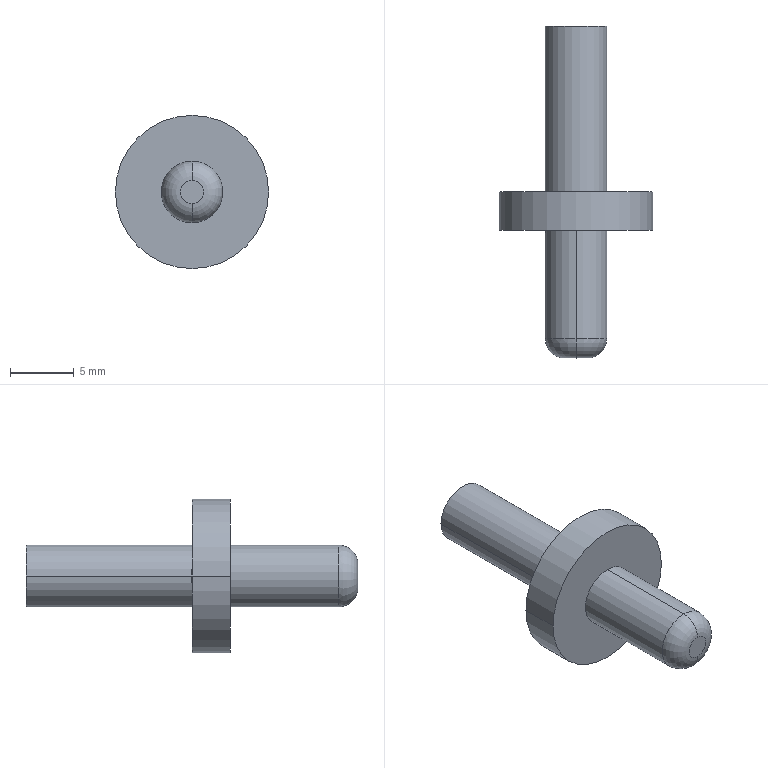Part | SolidWorks | features BaseBody 1 | 1 solid | 12 faces | box 12 x 26 x 12 mm | volume 754.399 mm3 | cylinder 6 | plane 4 | torus 2 | commonest cylinder face diameters 4.83 x4 12 x2
STEP:
#1=CARTESIAN_POINT('',(0.,1.5,-2.415));
#2=VERTEX_POINT('',#1);
#3=CARTESIAN_POINT('',(0.,1.5,2.415));
#4=VERTEX_POINT('',#3);
#5=CARTESIAN_POINT('',(0.,1.5,0.));
#6=DIRECTION('',(0.,-1.,0.));
#7=DIRECTION('',(0.,0.,-1.));
#8=AXIS2_PLACEMENT_3D('',#5,#6,#7);
#9=CIRCLE('',#8,2.415);
#10=EDGE_CURVE('',#2,#4,#9,.T.);
#11=ORIENTED_EDGE('',*,*,#10,.T.);
#12=CARTESIAN_POINT('',(0.,0.,0.915));
#13=VERTEX_POINT('',#12);
#14=CARTESIAN_POINT('',(0.,1.5,0.915));
#15=DIRECTION('',(1.,0.,0.));
#16=DIRECTION('',(0.,0.,-1.));
#17=AXIS2_PLACEMENT_3D('',#14,#15,#16);
#18=CIRCLE('',#17,1.5);
#19=EDGE_CURVE('',#4,#13,#18,.T.);
#20=ORIENTED_EDGE('',*,*,#19,.T.);
#21=CARTESIAN_POINT('',(0.,0.,-0.915));
#22=VERTEX_POINT('',#21);
#23=CARTESIAN_POINT('',(0.,0.,0.));
#24=DIRECTION('',(0.,1.,0.));
#25=DIRECTION('',(0.,0.,-1.));
#26=AXIS2_PLACEMENT_3D('',#23,#24,#25);
#27=CIRCLE('',#26,0.915);
#28=EDGE_CURVE('',#13,#22,#27,.T.);
#29=ORIENTED_EDGE('',*,*,#28,.T.);
#30=CARTESIAN_POINT('',(0.,1.5,-0.915));
#31=DIRECTION('',(-1.,0.,0.));
#32=DIRECTION('',(0.,0.,1.));
#33=AXIS2_PLACEMENT_3D('',#30,#31,#32);
#34=CIRCLE('',#33,1.5);
#35=EDGE_CURVE('',#2,#22,#34,.T.);
#36=ORIENTED_EDGE('',*,*,#35,.F.);
#37=EDGE_LOOP('',(#11,#20,#29,#36));
#38=FACE_OUTER_BOUND('',#37,.T.);
#39=CARTESIAN_POINT('',(0.,1.5,0.));
#40=DIRECTION('',(0.,-1.,0.));
#41=DIRECTION('',(0.,0.,-1.));
#42=AXIS2_PLACEMENT_3D('',#39,#40,#41);
#43=TOROIDAL_SURFACE('',#42,0.915,1.5);
#44=ADVANCED_FACE('',(#38),#43,.T.);
#45=ORIENTED_EDGE('',*,*,#10,.F.);
#46=CARTESIAN_POINT('',(0.,10.,-2.415));
#47=VERTEX_POINT('',#46);
#48=CARTESIAN_POINT('',(0.,1.5,-2.415));
#49=DIRECTION('',(0.,1.,0.));
#50=VECTOR('',#49,1000.);
#51=LINE('',#48,#50);
#52=EDGE_CURVE('',#2,#47,#51,.T.);
#53=ORIENTED_EDGE('',*,*,#52,.T.);
#54=CARTESIAN_POINT('',(0.,10.,2.415));
#55=VERTEX_POINT('',#54);
#56=CARTESIAN_POINT('',(0.,10.,0.));
#57=DIRECTION('',(0.,1.,0.));
#58=DIRECTION('',(0.,0.,1.));
#59=AXIS2_PLACEMENT_3D('',#56,#57,#58);
#60=CIRCLE('',#59,2.415);
#61=EDGE_CURVE('',#55,#47,#60,.T.);
#62=ORIENTED_EDGE('',*,*,#61,.F.);
#63=CARTESIAN_POINT('',(0.,1.5,2.415));
#64=DIRECTION('',(0.,1.,0.));
#65=VECTOR('',#64,1000.);
#66=LINE('',#63,#65);
#67=EDGE_CURVE('',#4,#55,#66,.T.);
#68=ORIENTED_EDGE('',*,*,#67,.F.);
#69=EDGE_LOOP('',(#45,#53,#62,#68));
#70=FACE_OUTER_BOUND('',#69,.T.);
#71=CARTESIAN_POINT('',(0.,1.5,0.));
#72=DIRECTION('',(0.,1.,0.));
#73=DIRECTION('',(0.,0.,1.));
#74=AXIS2_PLACEMENT_3D('',#71,#72,#73);
#75=CYLINDRICAL_SURFACE('',#74,2.415);
#76=ADVANCED_FACE('',(#70),#75,.T.);
#77=CARTESIAN_POINT('',(6.,10.,0.));
#78=VERTEX_POINT('',#77);
#79=CARTESIAN_POINT('',(-6.,10.,0.));
#80=VERTEX_POINT('',#79);
#81=CARTESIAN_POINT('',(0.,10.,0.));
#82=DIRECTION('',(0.,-1.,0.));
#83=DIRECTION('',(-1.,0.,0.));
#84=AXIS2_PLACEMENT_3D('',#81,#82,#83);
#85=CIRCLE('',#84,6.);
#86=EDGE_CURVE('',#78,#80,#85,.T.);
#87=ORIENTED_EDGE('',*,*,#86,.F.);
#88=CARTESIAN_POINT('',(6.,13.,0.));
#89=VERTEX_POINT('',#88);
#90=CARTESIAN_POINT('',(6.,10.,0.));
#91=DIRECTION('',(0.,1.,0.));
#92=VECTOR('',#91,1000.);
#93=LINE('',#90,#92);
#94=EDGE_CURVE('',#78,#89,#93,.T.);
#95=ORIENTED_EDGE('',*,*,#94,.T.);
#96=CARTESIAN_POINT('',(-6.,13.,0.));
#97=VERTEX_POINT('',#96);
#98=CARTESIAN_POINT('',(0.,13.,0.));
#99=DIRECTION('',(0.,1.,0.));
#100=DIRECTION('',(-1.,0.,0.));
#101=AXIS2_PLACEMENT_3D('',#98,#99,#100);
#102=CIRCLE('',#101,6.);
#103=EDGE_CURVE('',#97,#89,#102,.T.);
#104=ORIENTED_EDGE('',*,*,#103,.F.);
#105=CARTESIAN_POINT('',(-6.,10.,0.));
#106=DIRECTION('',(0.,1.,0.));
#107=VECTOR('',#106,1000.);
#108=LINE('',#105,#107);
#109=EDGE_CURVE('',#80,#97,#108,.T.);
#110=ORIENTED_EDGE('',*,*,#109,.F.);
#111=EDGE_LOOP('',(#87,#95,#104,#110));
#112=FACE_OUTER_BOUND('',#111,.T.);
#113=CARTESIAN_POINT('',(0.,10.,0.));
#114=DIRECTION('',(0.,1.,0.));
#115=DIRECTION('',(-1.,0.,0.));
#116=AXIS2_PLACEMENT_3D('',#113,#114,#115);
#117=CYLINDRICAL_SURFACE('',#116,6.);
#118=ADVANCED_FACE('',(#112),#117,.T.);
#119=CARTESIAN_POINT('',(2.415,13.,0.));
#120=VERTEX_POINT('',#119);
#121=CARTESIAN_POINT('',(-2.415,13.,0.));
#122=VERTEX_POINT('',#121);
#123=CARTESIAN_POINT('',(0.,13.,0.));
#124=DIRECTION('',(0.,-1.,0.));
#125=DIRECTION('',(-1.,0.,0.));
#126=AXIS2_PLACEMENT_3D('',#123,#124,#125);
#127=CIRCLE('',#126,2.415);
#128=EDGE_CURVE('',#120,#122,#127,.T.);
#129=ORIENTED_EDGE('',*,*,#128,.F.);
#130=CARTESIAN_POINT('',(2.415,26.,0.));
#131=VERTEX_POINT('',#130);
#132=CARTESIAN_POINT('',(2.415,13.,0.));
#133=DIRECTION('',(0.,1.,0.));
#134=VECTOR('',#133,1000.);
#135=LINE('',#132,#134);
#136=EDGE_CURVE('',#120,#131,#135,.T.);
#137=ORIENTED_EDGE('',*,*,#136,.T.);
#138=CARTESIAN_POINT('',(-2.415,26.,0.));
#139=VERTEX_POINT('',#138);
#140=CARTESIAN_POINT('',(0.,26.,0.));
#141=DIRECTION('',(0.,1.,0.));
#142=DIRECTION('',(-1.,0.,0.));
#143=AXIS2_PLACEMENT_3D('',#140,#141,#142);
#144=CIRCLE('',#143,2.415);
#145=EDGE_CURVE('',#139,#131,#144,.T.);
#146=ORIENTED_EDGE('',*,*,#145,.F.);
#147=CARTESIAN_POINT('',(-2.415,13.,0.));
#148=DIRECTION('',(0.,1.,0.));
#149=VECTOR('',#148,1000.);
#150=LINE('',#147,#149);
#151=EDGE_CURVE('',#122,#139,#150,.T.);
#152=ORIENTED_EDGE('',*,*,#151,.F.);
#153=EDGE_LOOP('',(#129,#137,#146,#152));
#154=FACE_OUTER_BOUND('',#153,.T.);
#155=CARTESIAN_POINT('',(0.,13.,0.));
#156=DIRECTION('',(0.,1.,0.));
#157=DIRECTION('',(-1.,0.,0.));
#158=AXIS2_PLACEMENT_3D('',#155,#156,#157);
#159=CYLINDRICAL_SURFACE('',#158,2.415);
#160=ADVANCED_FACE('',(#154),#159,.T.);
#161=ORIENTED_EDGE('',*,*,#19,.F.);
#162=CARTESIAN_POINT('',(0.,1.5,0.));
#163=DIRECTION('',(0.,-1.,0.));
#164=DIRECTION('',(0.,0.,-1.));
#165=AXIS2_PLACEMENT_3D('',#162,#163,#164);
#166=CIRCLE('',#165,2.415);
#167=EDGE_CURVE('',#4,#2,#166,.T.);
#168=ORIENTED_EDGE('',*,*,#167,.T.);
#169=ORIENTED_EDGE('',*,*,#35,.T.);
#170=CARTESIAN_POINT('',(0.,0.,0.));
#171=DIRECTION('',(0.,1.,0.));
#172=DIRECTION('',(0.,0.,-1.));
#173=AXIS2_PLACEMENT_3D('',#170,#171,#172);
#174=CIRCLE('',#173,0.915);
#175=EDGE_CURVE('',#22,#13,#174,.T.);
#176=ORIENTED_EDGE('',*,*,#175,.T.);
#177=EDGE_LOOP('',(#161,#168,#169,#176));
#178=FACE_OUTER_BOUND('',#177,.T.);
#179=CARTESIAN_POINT('',(0.,1.5,0.));
#180=DIRECTION('',(0.,-1.,0.));
#181=DIRECTION('',(0.,0.,-1.));
#182=AXIS2_PLACEMENT_3D('',#179,#180,#181);
#183=TOROIDAL_SURFACE('',#182,0.915,1.5);
#184=ADVANCED_FACE('',(#178),#183,.T.);
#185=ORIENTED_EDGE('',*,*,#175,.F.);
#186=ORIENTED_EDGE('',*,*,#28,.F.);
#187=EDGE_LOOP('',(#185,#186));
#188=FACE_OUTER_BOUND('',#187,.T.);
#189=CARTESIAN_POINT('',(-0.926,0.,0.926));
#190=DIRECTION('',(0.,-1.,0.));
#191=DIRECTION('',(0.,0.,-1.));
#192=AXIS2_PLACEMENT_3D('',#189,#190,#191);
#193=PLANE('',#192);
#194=ADVANCED_FACE('',(#188),#193,.T.);
#195=ORIENTED_EDGE('',*,*,#52,.F.);
#196=ORIENTED_EDGE('',*,*,#167,.F.);
#197=ORIENTED_EDGE('',*,*,#67,.T.);
#198=CARTESIAN_POINT('',(0.,10.,0.));
#199=DIRECTION('',(0.,1.,0.));
#200=DIRECTION('',(0.,0.,1.));
#201=AXIS2_PLACEMENT_3D('',#198,#199,#200);
#202=CIRCLE('',#201,2.415);
#203=EDGE_CURVE('',#47,#55,#202,.T.);
#204=ORIENTED_EDGE('',*,*,#203,.F.);
#205=EDGE_LOOP('',(#195,#196,#197,#204));
#206=FACE_OUTER_BOUND('',#205,.T.);
#207=CARTESIAN_POINT('',(0.,1.5,0.));
#208=DIRECTION('',(0.,1.,0.));
#209=DIRECTION('',(0.,0.,1.));
#210=AXIS2_PLACEMENT_3D('',#207,#208,#209);
#211=CYLINDRICAL_SURFACE('',#210,2.415);
#212=ADVANCED_FACE('',(#206),#211,.T.);
#213=ORIENTED_EDGE('',*,*,#61,.T.);
#214=ORIENTED_EDGE('',*,*,#203,.T.);
#215=EDGE_LOOP('',(#213,#214));
#216=FACE_BOUND('',#215,.T.);
#217=CARTESIAN_POINT('',(0.,10.,0.));
#218=DIRECTION('',(0.,-1.,0.));
#219=DIRECTION('',(-1.,0.,0.));
#220=AXIS2_PLACEMENT_3D('',#217,#218,#219);
#221=CIRCLE('',#220,6.);
#222=EDGE_CURVE('',#80,#78,#221,.T.);
#223=ORIENTED_EDGE('',*,*,#222,.T.);
#224=ORIENTED_EDGE('',*,*,#86,.T.);
#225=EDGE_LOOP('',(#223,#224));
#226=FACE_OUTER_BOUND('',#225,.T.);
#227=CARTESIAN_POINT('',(-6.072,10.,6.072));
#228=DIRECTION('',(0.,-1.,0.));
#229=DIRECTION('',(0.,0.,-1.));
#230=AXIS2_PLACEMENT_3D('',#227,#228,#229);
#231=PLANE('',#230);
#232=ADVANCED_FACE('',(#216,#226),#231,.T.);
#233=ORIENTED_EDGE('',*,*,#94,.F.);
#234=ORIENTED_EDGE('',*,*,#222,.F.);
#235=ORIENTED_EDGE('',*,*,#109,.T.);
#236=CARTESIAN_POINT('',(0.,13.,0.));
#237=DIRECTION('',(0.,1.,0.));
#238=DIRECTION('',(-1.,0.,0.));
#239=AXIS2_PLACEMENT_3D('',#236,#237,#238);
#240=CIRCLE('',#239,6.);
#241=EDGE_CURVE('',#89,#97,#240,.T.);
#242=ORIENTED_EDGE('',*,*,#241,.F.);
#243=EDGE_LOOP('',(#233,#234,#235,#242));
#244=FACE_OUTER_BOUND('',#243,.T.);
#245=CARTESIAN_POINT('',(0.,10.,0.));
#246=DIRECTION('',(0.,1.,0.));
#247=DIRECTION('',(-1.,0.,0.));
#248=AXIS2_PLACEMENT_3D('',#245,#246,#247);
#249=CYLINDRICAL_SURFACE('',#248,6.);
#250=ADVANCED_FACE('',(#244),#249,.T.);
#251=CARTESIAN_POINT('',(0.,13.,0.));
#252=DIRECTION('',(0.,-1.,0.));
#253=DIRECTION('',(-1.,0.,0.));
#254=AXIS2_PLACEMENT_3D('',#251,#252,#253);
#255=CIRCLE('',#254,2.415);
#256=EDGE_CURVE('',#122,#120,#255,.T.);
#257=ORIENTED_EDGE('',*,*,#256,.T.);
#258=ORIENTED_EDGE('',*,*,#128,.T.);
#259=EDGE_LOOP('',(#257,#258));
#260=FACE_BOUND('',#259,.T.);
#261=ORIENTED_EDGE('',*,*,#103,.T.);
#262=ORIENTED_EDGE('',*,*,#241,.T.);
#263=EDGE_LOOP('',(#261,#262));
#264=FACE_OUTER_BOUND('',#263,.T.);
#265=CARTESIAN_POINT('',(-6.072,13.,-6.072));
#266=DIRECTION('',(0.,1.,0.));
#267=DIRECTION('',(0.,0.,1.));
#268=AXIS2_PLACEMENT_3D('',#265,#266,#267);
#269=PLANE('',#268);
#270=ADVANCED_FACE('',(#260,#264),#269,.T.);
#271=ORIENTED_EDGE('',*,*,#136,.F.);
#272=ORIENTED_EDGE('',*,*,#256,.F.);
#273=ORIENTED_EDGE('',*,*,#151,.T.);
#274=CARTESIAN_POINT('',(0.,26.,0.));
#275=DIRECTION('',(0.,1.,0.));
#276=DIRECTION('',(-1.,0.,0.));
#277=AXIS2_PLACEMENT_3D('',#274,#275,#276);
#278=CIRCLE('',#277,2.415);
#279=EDGE_CURVE('',#131,#139,#278,.T.);
#280=ORIENTED_EDGE('',*,*,#279,.F.);
#281=EDGE_LOOP('',(#271,#272,#273,#280));
#282=FACE_OUTER_BOUND('',#281,.T.);
#283=CARTESIAN_POINT('',(0.,13.,0.));
#284=DIRECTION('',(0.,1.,0.));
#285=DIRECTION('',(-1.,0.,0.));
#286=AXIS2_PLACEMENT_3D('',#283,#284,#285);
#287=CYLINDRICAL_SURFACE('',#286,2.415);
#288=ADVANCED_FACE('',(#282),#287,.T.);
#289=ORIENTED_EDGE('',*,*,#145,.T.);
#290=ORIENTED_EDGE('',*,*,#279,.T.);
#291=EDGE_LOOP('',(#289,#290));
#292=FACE_OUTER_BOUND('',#291,.T.);
#293=CARTESIAN_POINT('',(-2.444,26.,-2.444));
#294=DIRECTION('',(0.,1.,0.));
#295=DIRECTION('',(0.,0.,1.));
#296=AXIS2_PLACEMENT_3D('',#293,#294,#295);
#297=PLANE('',#296);
#298=ADVANCED_FACE('',(#292),#297,.T.);
#299=CLOSED_SHELL('',(#44,#76,#118,#160,#184,#194,#212,#232,#250,#270,#288,#298));
#300=MANIFOLD_SOLID_BREP('',#299);
#301=CARTESIAN_POINT('',(0.,0.,0.));
#302=DIRECTION('',(0.,0.,1.));
#303=DIRECTION('',(1.,0.,0.));
#304=AXIS2_PLACEMENT_3D('',#301,#302,#303);
#305=(LENGTH_UNIT()NAMED_UNIT(*)SI_UNIT(.MILLI.,.METRE.));
#306=UNCERTAINTY_MEASURE_WITH_UNIT(LENGTH_MEASURE(0.00001),#305,'','');
#307=(NAMED_UNIT(*)PLANE_ANGLE_UNIT()SI_UNIT($,.RADIAN.));
#308=(NAMED_UNIT(*)SI_UNIT($,.STERADIAN.)SOLID_ANGLE_UNIT());
#309=(GEOMETRIC_REPRESENTATION_CONTEXT(3)GLOBAL_UNCERTAINTY_ASSIGNED_CONTEXT((#306))GLOBAL_UNIT_ASSIGNED_CONTEXT((#305,#307,#308))REPRESENTATION_CONTEXT('',''));
#310=ADVANCED_BREP_SHAPE_REPRESENTATION('',(#300,#304),#309);